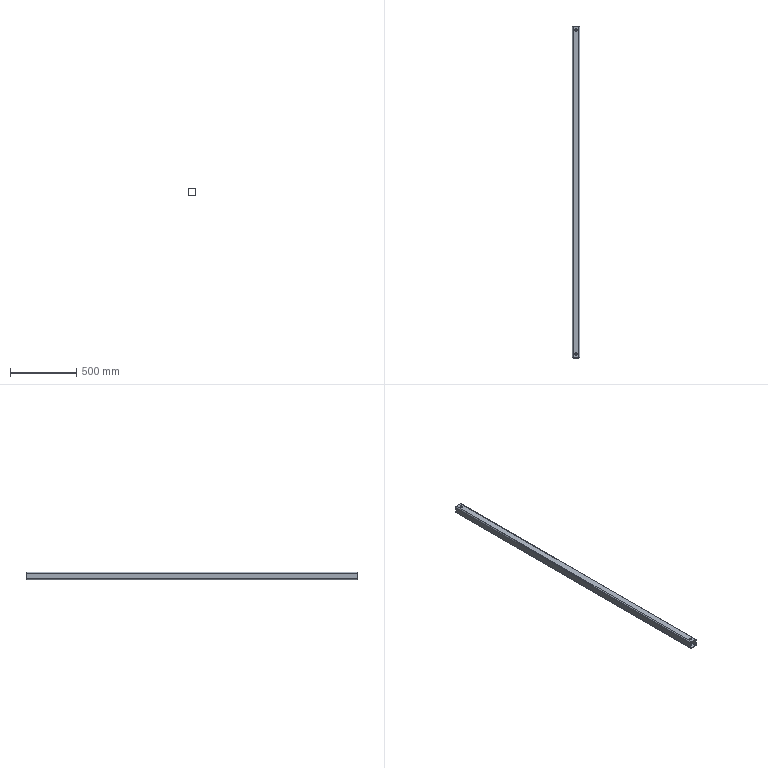Part | SolidWorks | features BaseBody 1 | 1 solid | 26 faces | box 60 x 2500 x 60 mm | volume 2133143 mm3 | cylinder 16 | plane 10 | commonest cylinder face diameters 17.5 x8 8 x4 16 x4
STEP:
#1=CARTESIAN_POINT('',(-678.75,22.,-1300.));
#2=VERTEX_POINT('',#1);
#3=CARTESIAN_POINT('',(-661.25,22.,-1300.));
#4=VERTEX_POINT('',#3);
#5=CARTESIAN_POINT('',(-670.,22.,-1300.));
#6=DIRECTION('',(0.,0.,1.));
#7=DIRECTION('',(-1.,0.,0.));
#8=AXIS2_PLACEMENT_3D('',#5,#6,#7);
#9=CIRCLE('',#8,8.75);
#10=EDGE_CURVE('',#2,#4,#9,.T.);
#11=ORIENTED_EDGE('',*,*,#10,.T.);
#12=CARTESIAN_POINT('',(-661.25,22.,-1304.));
#13=VERTEX_POINT('',#12);
#14=CARTESIAN_POINT('',(-661.25,22.,-1580.));
#15=DIRECTION('',(0.,0.,-1.));
#16=VECTOR('',#15,1000.);
#17=LINE('',#14,#16);
#18=EDGE_CURVE('',#4,#13,#17,.T.);
#19=ORIENTED_EDGE('',*,*,#18,.T.);
#20=CARTESIAN_POINT('',(-678.75,22.,-1304.));
#21=VERTEX_POINT('',#20);
#22=CARTESIAN_POINT('',(-670.,22.,-1304.));
#23=DIRECTION('',(0.,0.,1.));
#24=DIRECTION('',(-1.,0.,0.));
#25=AXIS2_PLACEMENT_3D('',#22,#23,#24);
#26=CIRCLE('',#25,8.75);
#27=EDGE_CURVE('',#21,#13,#26,.T.);
#28=ORIENTED_EDGE('',*,*,#27,.F.);
#29=CARTESIAN_POINT('',(-678.75,22.,-1580.));
#30=DIRECTION('',(0.,0.,-1.));
#31=VECTOR('',#30,1000.);
#32=LINE('',#29,#31);
#33=EDGE_CURVE('',#2,#21,#32,.T.);
#34=ORIENTED_EDGE('',*,*,#33,.F.);
#35=EDGE_LOOP('',(#11,#19,#28,#34));
#36=FACE_OUTER_BOUND('',#35,.T.);
#37=CARTESIAN_POINT('',(-670.,22.,-1580.));
#38=DIRECTION('',(0.,0.,-1.));
#39=DIRECTION('',(-1.,0.,0.));
#40=AXIS2_PLACEMENT_3D('',#37,#38,#39);
#41=CYLINDRICAL_SURFACE('',#40,8.75);
#42=ADVANCED_FACE('',(#36),#41,.F.);
#43=CARTESIAN_POINT('',(-678.75,2462.,-1300.));
#44=VERTEX_POINT('',#43);
#45=CARTESIAN_POINT('',(-661.25,2462.,-1300.));
#46=VERTEX_POINT('',#45);
#47=CARTESIAN_POINT('',(-670.,2462.,-1300.));
#48=DIRECTION('',(0.,0.,1.));
#49=DIRECTION('',(-1.,0.,0.));
#50=AXIS2_PLACEMENT_3D('',#47,#48,#49);
#51=CIRCLE('',#50,8.75);
#52=EDGE_CURVE('',#44,#46,#51,.T.);
#53=ORIENTED_EDGE('',*,*,#52,.T.);
#54=CARTESIAN_POINT('',(-661.25,2462.,-1304.));
#55=VERTEX_POINT('',#54);
#56=CARTESIAN_POINT('',(-661.25,2462.,-1580.));
#57=DIRECTION('',(0.,0.,-1.));
#58=VECTOR('',#57,1000.);
#59=LINE('',#56,#58);
#60=EDGE_CURVE('',#46,#55,#59,.T.);
#61=ORIENTED_EDGE('',*,*,#60,.T.);
#62=CARTESIAN_POINT('',(-678.75,2462.,-1304.));
#63=VERTEX_POINT('',#62);
#64=CARTESIAN_POINT('',(-670.,2462.,-1304.));
#65=DIRECTION('',(0.,0.,1.));
#66=DIRECTION('',(-1.,0.,0.));
#67=AXIS2_PLACEMENT_3D('',#64,#65,#66);
#68=CIRCLE('',#67,8.75);
#69=EDGE_CURVE('',#63,#55,#68,.T.);
#70=ORIENTED_EDGE('',*,*,#69,.F.);
#71=CARTESIAN_POINT('',(-678.75,2462.,-1580.));
#72=DIRECTION('',(0.,0.,-1.));
#73=VECTOR('',#72,1000.);
#74=LINE('',#71,#73);
#75=EDGE_CURVE('',#44,#63,#74,.T.);
#76=ORIENTED_EDGE('',*,*,#75,.F.);
#77=EDGE_LOOP('',(#53,#61,#70,#76));
#78=FACE_OUTER_BOUND('',#77,.T.);
#79=CARTESIAN_POINT('',(-670.,2462.,-1580.));
#80=DIRECTION('',(0.,0.,-1.));
#81=DIRECTION('',(-1.,0.,0.));
#82=AXIS2_PLACEMENT_3D('',#79,#80,#81);
#83=CYLINDRICAL_SURFACE('',#82,8.75);
#84=ADVANCED_FACE('',(#78),#83,.F.);
#85=CARTESIAN_POINT('',(-661.25,22.,-1356.));
#86=VERTEX_POINT('',#85);
#87=CARTESIAN_POINT('',(-678.75,22.,-1356.));
#88=VERTEX_POINT('',#87);
#89=CARTESIAN_POINT('',(-670.,22.,-1356.));
#90=DIRECTION('',(0.,0.,-1.));
#91=DIRECTION('',(-1.,0.,0.));
#92=AXIS2_PLACEMENT_3D('',#89,#90,#91);
#93=CIRCLE('',#92,8.75);
#94=EDGE_CURVE('',#86,#88,#93,.T.);
#95=ORIENTED_EDGE('',*,*,#94,.F.);
#96=CARTESIAN_POINT('',(-661.25,22.,-1360.));
#97=VERTEX_POINT('',#96);
#98=CARTESIAN_POINT('',(-661.25,22.,-1580.));
#99=DIRECTION('',(0.,0.,-1.));
#100=VECTOR('',#99,1000.);
#101=LINE('',#98,#100);
#102=EDGE_CURVE('',#86,#97,#101,.T.);
#103=ORIENTED_EDGE('',*,*,#102,.T.);
#104=CARTESIAN_POINT('',(-678.75,22.,-1360.));
#105=VERTEX_POINT('',#104);
#106=CARTESIAN_POINT('',(-670.,22.,-1360.));
#107=DIRECTION('',(0.,0.,-1.));
#108=DIRECTION('',(-1.,0.,0.));
#109=AXIS2_PLACEMENT_3D('',#106,#107,#108);
#110=CIRCLE('',#109,8.75);
#111=EDGE_CURVE('',#97,#105,#110,.T.);
#112=ORIENTED_EDGE('',*,*,#111,.T.);
#113=CARTESIAN_POINT('',(-678.75,22.,-1580.));
#114=DIRECTION('',(0.,0.,-1.));
#115=VECTOR('',#114,1000.);
#116=LINE('',#113,#115);
#117=EDGE_CURVE('',#88,#105,#116,.T.);
#118=ORIENTED_EDGE('',*,*,#117,.F.);
#119=EDGE_LOOP('',(#95,#103,#112,#118));
#120=FACE_OUTER_BOUND('',#119,.T.);
#121=CARTESIAN_POINT('',(-670.,22.,-1580.));
#122=DIRECTION('',(0.,0.,-1.));
#123=DIRECTION('',(-1.,0.,0.));
#124=AXIS2_PLACEMENT_3D('',#121,#122,#123);
#125=CYLINDRICAL_SURFACE('',#124,8.75);
#126=ADVANCED_FACE('',(#120),#125,.F.);
#127=CARTESIAN_POINT('',(-661.25,2462.,-1356.));
#128=VERTEX_POINT('',#127);
#129=CARTESIAN_POINT('',(-678.75,2462.,-1356.));
#130=VERTEX_POINT('',#129);
#131=CARTESIAN_POINT('',(-670.,2462.,-1356.));
#132=DIRECTION('',(0.,0.,-1.));
#133=DIRECTION('',(-1.,0.,0.));
#134=AXIS2_PLACEMENT_3D('',#131,#132,#133);
#135=CIRCLE('',#134,8.75);
#136=EDGE_CURVE('',#128,#130,#135,.T.);
#137=ORIENTED_EDGE('',*,*,#136,.F.);
#138=CARTESIAN_POINT('',(-661.25,2462.,-1360.));
#139=VERTEX_POINT('',#138);
#140=CARTESIAN_POINT('',(-661.25,2462.,-1580.));
#141=DIRECTION('',(0.,0.,-1.));
#142=VECTOR('',#141,1000.);
#143=LINE('',#140,#142);
#144=EDGE_CURVE('',#128,#139,#143,.T.);
#145=ORIENTED_EDGE('',*,*,#144,.T.);
#146=CARTESIAN_POINT('',(-678.75,2462.,-1360.));
#147=VERTEX_POINT('',#146);
#148=CARTESIAN_POINT('',(-670.,2462.,-1360.));
#149=DIRECTION('',(0.,0.,-1.));
#150=DIRECTION('',(-1.,0.,0.));
#151=AXIS2_PLACEMENT_3D('',#148,#149,#150);
#152=CIRCLE('',#151,8.75);
#153=EDGE_CURVE('',#139,#147,#152,.T.);
#154=ORIENTED_EDGE('',*,*,#153,.T.);
#155=CARTESIAN_POINT('',(-678.75,2462.,-1580.));
#156=DIRECTION('',(0.,0.,-1.));
#157=VECTOR('',#156,1000.);
#158=LINE('',#155,#157);
#159=EDGE_CURVE('',#130,#147,#158,.T.);
#160=ORIENTED_EDGE('',*,*,#159,.F.);
#161=EDGE_LOOP('',(#137,#145,#154,#160));
#162=FACE_OUTER_BOUND('',#161,.T.);
#163=CARTESIAN_POINT('',(-670.,2462.,-1580.));
#164=DIRECTION('',(0.,0.,-1.));
#165=DIRECTION('',(-1.,0.,0.));
#166=AXIS2_PLACEMENT_3D('',#163,#164,#165);
#167=CYLINDRICAL_SURFACE('',#166,8.75);
#168=ADVANCED_FACE('',(#162),#167,.F.);
#169=CARTESIAN_POINT('',(-696.,2492.,-1352.));
#170=VERTEX_POINT('',#169);
#171=CARTESIAN_POINT('',(-696.,2492.,-1308.));
#172=VERTEX_POINT('',#171);
#173=CARTESIAN_POINT('',(-696.,2492.,-1308.));
#174=DIRECTION('',(0.,0.,1.));
#175=VECTOR('',#174,1000.);
#176=LINE('',#173,#175);
#177=EDGE_CURVE('',#170,#172,#176,.T.);
#178=ORIENTED_EDGE('',*,*,#177,.T.);
#179=CARTESIAN_POINT('',(-696.,-8.,-1308.));
#180=VERTEX_POINT('',#179);
#181=CARTESIAN_POINT('',(-696.,22.,-1308.));
#182=DIRECTION('',(0.,-1.,0.));
#183=VECTOR('',#182,1000.);
#184=LINE('',#181,#183);
#185=EDGE_CURVE('',#172,#180,#184,.T.);
#186=ORIENTED_EDGE('',*,*,#185,.T.);
#187=CARTESIAN_POINT('',(-696.,-8.,-1352.));
#188=VERTEX_POINT('',#187);
#189=CARTESIAN_POINT('',(-696.,-8.,-1308.));
#190=DIRECTION('',(0.,0.,-1.));
#191=VECTOR('',#190,1000.);
#192=LINE('',#189,#191);
#193=EDGE_CURVE('',#180,#188,#192,.T.);
#194=ORIENTED_EDGE('',*,*,#193,.T.);
#195=CARTESIAN_POINT('',(-696.,22.,-1352.));
#196=DIRECTION('',(0.,1.,0.));
#197=VECTOR('',#196,1000.);
#198=LINE('',#195,#197);
#199=EDGE_CURVE('',#188,#170,#198,.T.);
#200=ORIENTED_EDGE('',*,*,#199,.T.);
#201=EDGE_LOOP('',(#178,#186,#194,#200));
#202=FACE_OUTER_BOUND('',#201,.T.);
#203=CARTESIAN_POINT('',(-696.,22.,-1308.));
#204=DIRECTION('',(1.,0.,0.));
#205=DIRECTION('',(0.,0.,-1.));
#206=AXIS2_PLACEMENT_3D('',#203,#204,#205);
#207=PLANE('',#206);
#208=ADVANCED_FACE('',(#202),#207,.T.);
#209=ORIENTED_EDGE('',*,*,#185,.F.);
#210=CARTESIAN_POINT('',(-692.,2492.,-1304.));
#211=VERTEX_POINT('',#210);
#212=CARTESIAN_POINT('',(-692.,2492.,-1308.));
#213=DIRECTION('',(0.,-1.,0.));
#214=DIRECTION('',(0.,0.,1.));
#215=AXIS2_PLACEMENT_3D('',#212,#213,#214);
#216=CIRCLE('',#215,4.);
#217=EDGE_CURVE('',#211,#172,#216,.T.);
#218=ORIENTED_EDGE('',*,*,#217,.F.);
#219=CARTESIAN_POINT('',(-692.,-8.,-1304.));
#220=VERTEX_POINT('',#219);
#221=CARTESIAN_POINT('',(-692.,22.,-1304.));
#222=DIRECTION('',(0.,1.,0.));
#223=VECTOR('',#222,1000.);
#224=LINE('',#221,#223);
#225=EDGE_CURVE('',#220,#211,#224,.T.);
#226=ORIENTED_EDGE('',*,*,#225,.F.);
#227=CARTESIAN_POINT('',(-692.,-8.,-1308.));
#228=DIRECTION('',(0.,1.,0.));
#229=DIRECTION('',(0.,0.,1.));
#230=AXIS2_PLACEMENT_3D('',#227,#228,#229);
#231=CIRCLE('',#230,4.);
#232=EDGE_CURVE('',#180,#220,#231,.T.);
#233=ORIENTED_EDGE('',*,*,#232,.F.);
#234=EDGE_LOOP('',(#209,#218,#226,#233));
#235=FACE_OUTER_BOUND('',#234,.T.);
#236=CARTESIAN_POINT('',(-692.,22.,-1308.));
#237=DIRECTION('',(0.,1.,0.));
#238=DIRECTION('',(0.,0.,1.));
#239=AXIS2_PLACEMENT_3D('',#236,#237,#238);
#240=CYLINDRICAL_SURFACE('',#239,4.);
#241=ADVANCED_FACE('',(#235),#240,.F.);
#242=CARTESIAN_POINT('',(-692.,2492.,-1356.));
#243=VERTEX_POINT('',#242);
#244=CARTESIAN_POINT('',(-692.,2492.,-1352.));
#245=DIRECTION('',(0.,-1.,0.));
#246=DIRECTION('',(0.,0.,1.));
#247=AXIS2_PLACEMENT_3D('',#244,#245,#246);
#248=CIRCLE('',#247,4.);
#249=EDGE_CURVE('',#170,#243,#248,.T.);
#250=ORIENTED_EDGE('',*,*,#249,.T.);
#251=CARTESIAN_POINT('',(-648.,2492.,-1356.));
#252=VERTEX_POINT('',#251);
#253=CARTESIAN_POINT('',(-670.,2492.,-1356.));
#254=DIRECTION('',(1.,0.,0.));
#255=VECTOR('',#254,1000.);
#256=LINE('',#253,#255);
#257=EDGE_CURVE('',#243,#252,#256,.T.);
#258=ORIENTED_EDGE('',*,*,#257,.T.);
#259=CARTESIAN_POINT('',(-644.,2492.,-1352.));
#260=VERTEX_POINT('',#259);
#261=CARTESIAN_POINT('',(-648.,2492.,-1352.));
#262=DIRECTION('',(0.,-1.,0.));
#263=DIRECTION('',(0.,0.,1.));
#264=AXIS2_PLACEMENT_3D('',#261,#262,#263);
#265=CIRCLE('',#264,4.);
#266=EDGE_CURVE('',#252,#260,#265,.T.);
#267=ORIENTED_EDGE('',*,*,#266,.T.);
#268=CARTESIAN_POINT('',(-644.,2492.,-1308.));
#269=VERTEX_POINT('',#268);
#270=CARTESIAN_POINT('',(-644.,2492.,-1445.));
#271=DIRECTION('',(0.,0.,1.));
#272=VECTOR('',#271,1000.);
#273=LINE('',#270,#272);
#274=EDGE_CURVE('',#260,#269,#273,.T.);
#275=ORIENTED_EDGE('',*,*,#274,.T.);
#276=CARTESIAN_POINT('',(-648.,2492.,-1304.));
#277=VERTEX_POINT('',#276);
#278=CARTESIAN_POINT('',(-648.,2492.,-1308.));
#279=DIRECTION('',(0.,-1.,0.));
#280=DIRECTION('',(0.,0.,1.));
#281=AXIS2_PLACEMENT_3D('',#278,#279,#280);
#282=CIRCLE('',#281,4.);
#283=EDGE_CURVE('',#269,#277,#282,.T.);
#284=ORIENTED_EDGE('',*,*,#283,.T.);
#285=CARTESIAN_POINT('',(-670.,2492.,-1304.));
#286=DIRECTION('',(-1.,0.,0.));
#287=VECTOR('',#286,1000.);
#288=LINE('',#285,#287);
#289=EDGE_CURVE('',#277,#211,#288,.T.);
#290=ORIENTED_EDGE('',*,*,#289,.T.);
#291=ORIENTED_EDGE('',*,*,#217,.T.);
#292=ORIENTED_EDGE('',*,*,#177,.F.);
#293=EDGE_LOOP('',(#250,#258,#267,#275,#284,#290,#291,#292));
#294=FACE_BOUND('',#293,.T.);
#295=CARTESIAN_POINT('',(-700.,2492.,-1352.));
#296=VERTEX_POINT('',#295);
#297=CARTESIAN_POINT('',(-700.,2492.,-1308.));
#298=VERTEX_POINT('',#297);
#299=CARTESIAN_POINT('',(-700.,2492.,-1445.));
#300=DIRECTION('',(0.,0.,1.));
#301=VECTOR('',#300,1000.);
#302=LINE('',#299,#301);
#303=EDGE_CURVE('',#296,#298,#302,.T.);
#304=ORIENTED_EDGE('',*,*,#303,.T.);
#305=CARTESIAN_POINT('',(-692.,2492.,-1300.));
#306=VERTEX_POINT('',#305);
#307=CARTESIAN_POINT('',(-692.,2492.,-1308.));
#308=DIRECTION('',(0.,1.,0.));
#309=DIRECTION('',(0.,0.,1.));
#310=AXIS2_PLACEMENT_3D('',#307,#308,#309);
#311=CIRCLE('',#310,8.);
#312=EDGE_CURVE('',#298,#306,#311,.T.);
#313=ORIENTED_EDGE('',*,*,#312,.T.);
#314=CARTESIAN_POINT('',(-648.,2492.,-1300.));
#315=VERTEX_POINT('',#314);
#316=CARTESIAN_POINT('',(-670.,2492.,-1300.));
#317=DIRECTION('',(1.,0.,0.));
#318=VECTOR('',#317,1000.);
#319=LINE('',#316,#318);
#320=EDGE_CURVE('',#306,#315,#319,.T.);
#321=ORIENTED_EDGE('',*,*,#320,.T.);
#322=CARTESIAN_POINT('',(-640.,2492.,-1308.));
#323=VERTEX_POINT('',#322);
#324=CARTESIAN_POINT('',(-648.,2492.,-1308.));
#325=DIRECTION('',(0.,1.,0.));
#326=DIRECTION('',(0.,0.,1.));
#327=AXIS2_PLACEMENT_3D('',#324,#325,#326);
#328=CIRCLE('',#327,8.);
#329=EDGE_CURVE('',#315,#323,#328,.T.);
#330=ORIENTED_EDGE('',*,*,#329,.T.);
#331=CARTESIAN_POINT('',(-640.,2492.,-1352.));
#332=VERTEX_POINT('',#331);
#333=CARTESIAN_POINT('',(-640.,2492.,-1445.));
#334=DIRECTION('',(0.,0.,-1.));
#335=VECTOR('',#334,1000.);
#336=LINE('',#333,#335);
#337=EDGE_CURVE('',#323,#332,#336,.T.);
#338=ORIENTED_EDGE('',*,*,#337,.T.);
#339=CARTESIAN_POINT('',(-648.,2492.,-1360.));
#340=VERTEX_POINT('',#339);
#341=CARTESIAN_POINT('',(-648.,2492.,-1352.));
#342=DIRECTION('',(0.,1.,0.));
#343=DIRECTION('',(0.,0.,1.));
#344=AXIS2_PLACEMENT_3D('',#341,#342,#343);
#345=CIRCLE('',#344,8.);
#346=EDGE_CURVE('',#332,#340,#345,.T.);
#347=ORIENTED_EDGE('',*,*,#346,.T.);
#348=CARTESIAN_POINT('',(-692.,2492.,-1360.));
#349=VERTEX_POINT('',#348);
#350=CARTESIAN_POINT('',(-670.,2492.,-1360.));
#351=DIRECTION('',(-1.,0.,0.));
#352=VECTOR('',#351,1000.);
#353=LINE('',#350,#352);
#354=EDGE_CURVE('',#340,#349,#353,.T.);
#355=ORIENTED_EDGE('',*,*,#354,.T.);
#356=CARTESIAN_POINT('',(-692.,2492.,-1352.));
#357=DIRECTION('',(0.,1.,0.));
#358=DIRECTION('',(0.,0.,1.));
#359=AXIS2_PLACEMENT_3D('',#356,#357,#358);
#360=CIRCLE('',#359,8.);
#361=EDGE_CURVE('',#349,#296,#360,.T.);
#362=ORIENTED_EDGE('',*,*,#361,.T.);
#363=EDGE_LOOP('',(#304,#313,#321,#330,#338,#347,#355,#362));
#364=FACE_OUTER_BOUND('',#363,.T.);
#365=CARTESIAN_POINT('',(-670.,2492.,-1445.));
#366=DIRECTION('',(0.,1.,0.));
#367=DIRECTION('',(0.,0.,1.));
#368=AXIS2_PLACEMENT_3D('',#365,#366,#367);
#369=PLANE('',#368);
#370=ADVANCED_FACE('',(#294,#364),#369,.T.);
#371=CARTESIAN_POINT('',(-692.,-8.,-1356.));
#372=VERTEX_POINT('',#371);
#373=CARTESIAN_POINT('',(-692.,22.,-1356.));
#374=DIRECTION('',(0.,-1.,0.));
#375=VECTOR('',#374,1000.);
#376=LINE('',#373,#375);
#377=EDGE_CURVE('',#243,#372,#376,.T.);
#378=ORIENTED_EDGE('',*,*,#377,.F.);
#379=ORIENTED_EDGE('',*,*,#249,.F.);
#380=ORIENTED_EDGE('',*,*,#199,.F.);
#381=CARTESIAN_POINT('',(-692.,-8.,-1352.));
#382=DIRECTION('',(0.,1.,0.));
#383=DIRECTION('',(0.,0.,1.));
#384=AXIS2_PLACEMENT_3D('',#381,#382,#383);
#385=CIRCLE('',#384,4.);
#386=EDGE_CURVE('',#372,#188,#385,.T.);
#387=ORIENTED_EDGE('',*,*,#386,.F.);
#388=EDGE_LOOP('',(#378,#379,#380,#387));
#389=FACE_OUTER_BOUND('',#388,.T.);
#390=CARTESIAN_POINT('',(-692.,22.,-1352.));
#391=DIRECTION('',(0.,1.,0.));
#392=DIRECTION('',(0.,0.,1.));
#393=AXIS2_PLACEMENT_3D('',#390,#391,#392);
#394=CYLINDRICAL_SURFACE('',#393,4.);
#395=ADVANCED_FACE('',(#389),#394,.F.);
#396=CARTESIAN_POINT('',(-644.,-8.,-1352.));
#397=VERTEX_POINT('',#396);
#398=CARTESIAN_POINT('',(-648.,-8.,-1356.));
#399=VERTEX_POINT('',#398);
#400=CARTESIAN_POINT('',(-648.,-8.,-1352.));
#401=DIRECTION('',(0.,1.,0.));
#402=DIRECTION('',(0.,0.,1.));
#403=AXIS2_PLACEMENT_3D('',#400,#401,#402);
#404=CIRCLE('',#403,4.);
#405=EDGE_CURVE('',#397,#399,#404,.T.);
#406=ORIENTED_EDGE('',*,*,#405,.T.);
#407=CARTESIAN_POINT('',(-670.,-8.,-1356.));
#408=DIRECTION('',(-1.,0.,0.));
#409=VECTOR('',#408,1000.);
#410=LINE('',#407,#409);
#411=EDGE_CURVE('',#399,#372,#410,.T.);
#412=ORIENTED_EDGE('',*,*,#411,.T.);
#413=ORIENTED_EDGE('',*,*,#386,.T.);
#414=ORIENTED_EDGE('',*,*,#193,.F.);
#415=ORIENTED_EDGE('',*,*,#232,.T.);
#416=CARTESIAN_POINT('',(-648.,-8.,-1304.));
#417=VERTEX_POINT('',#416);
#418=CARTESIAN_POINT('',(-670.,-8.,-1304.));
#419=DIRECTION('',(1.,0.,0.));
#420=VECTOR('',#419,1000.);
#421=LINE('',#418,#420);
#422=EDGE_CURVE('',#220,#417,#421,.T.);
#423=ORIENTED_EDGE('',*,*,#422,.T.);
#424=CARTESIAN_POINT('',(-644.,-8.,-1308.));
#425=VERTEX_POINT('',#424);
#426=CARTESIAN_POINT('',(-648.,-8.,-1308.));
#427=DIRECTION('',(0.,1.,0.));
#428=DIRECTION('',(0.,0.,1.));
#429=AXIS2_PLACEMENT_3D('',#426,#427,#428);
#430=CIRCLE('',#429,4.);
#431=EDGE_CURVE('',#417,#425,#430,.T.);
#432=ORIENTED_EDGE('',*,*,#431,.T.);
#433=CARTESIAN_POINT('',(-644.,-8.,-1445.));
#434=DIRECTION('',(0.,0.,-1.));
#435=VECTOR('',#434,1000.);
#436=LINE('',#433,#435);
#437=EDGE_CURVE('',#425,#397,#436,.T.);
#438=ORIENTED_EDGE('',*,*,#437,.T.);
#439=EDGE_LOOP('',(#406,#412,#413,#414,#415,#423,#432,#438));
#440=FACE_BOUND('',#439,.T.);
#441=CARTESIAN_POINT('',(-640.,-8.,-1352.));
#442=VERTEX_POINT('',#441);
#443=CARTESIAN_POINT('',(-640.,-8.,-1308.));
#444=VERTEX_POINT('',#443);
#445=CARTESIAN_POINT('',(-640.,-8.,-1445.));
#446=DIRECTION('',(0.,0.,1.));
#447=VECTOR('',#446,1000.);
#448=LINE('',#445,#447);
#449=EDGE_CURVE('',#442,#444,#448,.T.);
#450=ORIENTED_EDGE('',*,*,#449,.T.);
#451=CARTESIAN_POINT('',(-648.,-8.,-1300.));
#452=VERTEX_POINT('',#451);
#453=CARTESIAN_POINT('',(-648.,-8.,-1308.));
#454=DIRECTION('',(0.,-1.,0.));
#455=DIRECTION('',(0.,0.,1.));
#456=AXIS2_PLACEMENT_3D('',#453,#454,#455);
#457=CIRCLE('',#456,8.);
#458=EDGE_CURVE('',#444,#452,#457,.T.);
#459=ORIENTED_EDGE('',*,*,#458,.T.);
#460=CARTESIAN_POINT('',(-692.,-8.,-1300.));
#461=VERTEX_POINT('',#460);
#462=CARTESIAN_POINT('',(-670.,-8.,-1300.));
#463=DIRECTION('',(-1.,0.,0.));
#464=VECTOR('',#463,1000.);
#465=LINE('',#462,#464);
#466=EDGE_CURVE('',#452,#461,#465,.T.);
#467=ORIENTED_EDGE('',*,*,#466,.T.);
#468=CARTESIAN_POINT('',(-700.,-8.,-1308.));
#469=VERTEX_POINT('',#468);
#470=CARTESIAN_POINT('',(-692.,-8.,-1308.));
#471=DIRECTION('',(0.,-1.,0.));
#472=DIRECTION('',(0.,0.,1.));
#473=AXIS2_PLACEMENT_3D('',#470,#471,#472);
#474=CIRCLE('',#473,8.);
#475=EDGE_CURVE('',#461,#469,#474,.T.);
#476=ORIENTED_EDGE('',*,*,#475,.T.);
#477=CARTESIAN_POINT('',(-700.,-8.,-1352.));
#478=VERTEX_POINT('',#477);
#479=CARTESIAN_POINT('',(-700.,-8.,-1445.));
#480=DIRECTION('',(0.,0.,-1.));
#481=VECTOR('',#480,1000.);
#482=LINE('',#479,#481);
#483=EDGE_CURVE('',#469,#478,#482,.T.);
#484=ORIENTED_EDGE('',*,*,#483,.T.);
#485=CARTESIAN_POINT('',(-692.,-8.,-1360.));
#486=VERTEX_POINT('',#485);
#487=CARTESIAN_POINT('',(-692.,-8.,-1352.));
#488=DIRECTION('',(0.,-1.,0.));
#489=DIRECTION('',(0.,0.,1.));
#490=AXIS2_PLACEMENT_3D('',#487,#488,#489);
#491=CIRCLE('',#490,8.);
#492=EDGE_CURVE('',#478,#486,#491,.T.);
#493=ORIENTED_EDGE('',*,*,#492,.T.);
#494=CARTESIAN_POINT('',(-648.,-8.,-1360.));
#495=VERTEX_POINT('',#494);
#496=CARTESIAN_POINT('',(-670.,-8.,-1360.));
#497=DIRECTION('',(1.,0.,0.));
#498=VECTOR('',#497,1000.);
#499=LINE('',#496,#498);
#500=EDGE_CURVE('',#486,#495,#499,.T.);
#501=ORIENTED_EDGE('',*,*,#500,.T.);
#502=CARTESIAN_POINT('',(-648.,-8.,-1352.));
#503=DIRECTION('',(0.,-1.,0.));
#504=DIRECTION('',(0.,0.,1.));
#505=AXIS2_PLACEMENT_3D('',#502,#503,#504);
#506=CIRCLE('',#505,8.);
#507=EDGE_CURVE('',#495,#442,#506,.T.);
#508=ORIENTED_EDGE('',*,*,#507,.T.);
#509=EDGE_LOOP('',(#450,#459,#467,#476,#484,#493,#501,#508));
#510=FACE_OUTER_BOUND('',#509,.T.);
#511=CARTESIAN_POINT('',(-670.,-8.,-1445.));
#512=DIRECTION('',(0.,-1.,0.));
#513=DIRECTION('',(0.,0.,-1.));
#514=AXIS2_PLACEMENT_3D('',#511,#512,#513);
#515=PLANE('',#514);
#516=ADVANCED_FACE('',(#440,#510),#515,.T.);
#517=ORIENTED_EDGE('',*,*,#27,.T.);
#518=CARTESIAN_POINT('',(-670.,22.,-1304.));
#519=DIRECTION('',(0.,0.,1.));
#520=DIRECTION('',(-1.,0.,0.));
#521=AXIS2_PLACEMENT_3D('',#518,#519,#520);
#522=CIRCLE('',#521,8.75);
#523=EDGE_CURVE('',#13,#21,#522,.T.);
#524=ORIENTED_EDGE('',*,*,#523,.T.);
#525=EDGE_LOOP('',(#517,#524));
#526=FACE_BOUND('',#525,.T.);
#527=ORIENTED_EDGE('',*,*,#69,.T.);
#528=CARTESIAN_POINT('',(-670.,2462.,-1304.));
#529=DIRECTION('',(0.,0.,1.));
#530=DIRECTION('',(-1.,0.,0.));
#531=AXIS2_PLACEMENT_3D('',#528,#529,#530);
#532=CIRCLE('',#531,8.75);
#533=EDGE_CURVE('',#55,#63,#532,.T.);
#534=ORIENTED_EDGE('',*,*,#533,.T.);
#535=EDGE_LOOP('',(#527,#534));
#536=FACE_BOUND('',#535,.T.);
#537=ORIENTED_EDGE('',*,*,#289,.F.);
#538=CARTESIAN_POINT('',(-648.,22.,-1304.));
#539=DIRECTION('',(0.,-1.,0.));
#540=VECTOR('',#539,1000.);
#541=LINE('',#538,#540);
#542=EDGE_CURVE('',#277,#417,#541,.T.);
#543=ORIENTED_EDGE('',*,*,#542,.T.);
#544=ORIENTED_EDGE('',*,*,#422,.F.);
#545=ORIENTED_EDGE('',*,*,#225,.T.);
#546=EDGE_LOOP('',(#537,#543,#544,#545));
#547=FACE_OUTER_BOUND('',#546,.T.);
#548=CARTESIAN_POINT('',(-692.,22.,-1304.));
#549=DIRECTION('',(0.,0.,-1.));
#550=DIRECTION('',(-1.,0.,0.));
#551=AXIS2_PLACEMENT_3D('',#548,#549,#550);
#552=PLANE('',#551);
#553=ADVANCED_FACE('',(#526,#536,#547),#552,.T.);
#554=CARTESIAN_POINT('',(-670.,22.,-1356.));
#555=DIRECTION('',(0.,0.,-1.));
#556=DIRECTION('',(-1.,0.,0.));
#557=AXIS2_PLACEMENT_3D('',#554,#555,#556);
#558=CIRCLE('',#557,8.75);
#559=EDGE_CURVE('',#88,#86,#558,.T.);
#560=ORIENTED_EDGE('',*,*,#559,.T.);
#561=ORIENTED_EDGE('',*,*,#94,.T.);
#562=EDGE_LOOP('',(#560,#561));
#563=FACE_BOUND('',#562,.T.);
#564=CARTESIAN_POINT('',(-670.,2462.,-1356.));
#565=DIRECTION('',(0.,0.,-1.));
#566=DIRECTION('',(-1.,0.,0.));
#567=AXIS2_PLACEMENT_3D('',#564,#565,#566);
#568=CIRCLE('',#567,8.75);
#569=EDGE_CURVE('',#130,#128,#568,.T.);
#570=ORIENTED_EDGE('',*,*,#569,.T.);
#571=ORIENTED_EDGE('',*,*,#136,.T.);
#572=EDGE_LOOP('',(#570,#571));
#573=FACE_BOUND('',#572,.T.);
#574=ORIENTED_EDGE('',*,*,#257,.F.);
#575=ORIENTED_EDGE('',*,*,#377,.T.);
#576=ORIENTED_EDGE('',*,*,#411,.F.);
#577=CARTESIAN_POINT('',(-648.,22.,-1356.));
#578=DIRECTION('',(0.,1.,0.));
#579=VECTOR('',#578,1000.);
#580=LINE('',#577,#579);
#581=EDGE_CURVE('',#399,#252,#580,.T.);
#582=ORIENTED_EDGE('',*,*,#581,.T.);
#583=EDGE_LOOP('',(#574,#575,#576,#582));
#584=FACE_OUTER_BOUND('',#583,.T.);
#585=CARTESIAN_POINT('',(-648.,22.,-1356.));
#586=DIRECTION('',(0.,0.,1.));
#587=DIRECTION('',(1.,0.,0.));
#588=AXIS2_PLACEMENT_3D('',#585,#586,#587);
#589=PLANE('',#588);
#590=ADVANCED_FACE('',(#563,#573,#584),#589,.T.);
#591=ORIENTED_EDGE('',*,*,#542,.F.);
#592=ORIENTED_EDGE('',*,*,#283,.F.);
#593=CARTESIAN_POINT('',(-644.,22.,-1308.));
#594=DIRECTION('',(0.,1.,0.));
#595=VECTOR('',#594,1000.);
#596=LINE('',#593,#595);
#597=EDGE_CURVE('',#425,#269,#596,.T.);
#598=ORIENTED_EDGE('',*,*,#597,.F.);
#599=ORIENTED_EDGE('',*,*,#431,.F.);
#600=EDGE_LOOP('',(#591,#592,#598,#599));
#601=FACE_OUTER_BOUND('',#600,.T.);
#602=CARTESIAN_POINT('',(-648.,22.,-1308.));
#603=DIRECTION('',(0.,1.,0.));
#604=DIRECTION('',(0.,0.,1.));
#605=AXIS2_PLACEMENT_3D('',#602,#603,#604);
#606=CYLINDRICAL_SURFACE('',#605,4.);
#607=ADVANCED_FACE('',(#601),#606,.F.);
#608=ORIENTED_EDGE('',*,*,#274,.F.);
#609=CARTESIAN_POINT('',(-644.,22.,-1352.));
#610=DIRECTION('',(0.,-1.,0.));
#611=VECTOR('',#610,1000.);
#612=LINE('',#609,#611);
#613=EDGE_CURVE('',#260,#397,#612,.T.);
#614=ORIENTED_EDGE('',*,*,#613,.T.);
#615=ORIENTED_EDGE('',*,*,#437,.F.);
#616=ORIENTED_EDGE('',*,*,#597,.T.);
#617=EDGE_LOOP('',(#608,#614,#615,#616));
#618=FACE_OUTER_BOUND('',#617,.T.);
#619=CARTESIAN_POINT('',(-644.,22.,-1352.));
#620=DIRECTION('',(-1.,0.,0.));
#621=DIRECTION('',(0.,0.,1.));
#622=AXIS2_PLACEMENT_3D('',#619,#620,#621);
#623=PLANE('',#622);
#624=ADVANCED_FACE('',(#618),#623,.T.);
#625=ORIENTED_EDGE('',*,*,#613,.F.);
#626=ORIENTED_EDGE('',*,*,#266,.F.);
#627=ORIENTED_EDGE('',*,*,#581,.F.);
#628=ORIENTED_EDGE('',*,*,#405,.F.);
#629=EDGE_LOOP('',(#625,#626,#627,#628));
#630=FACE_OUTER_BOUND('',#629,.T.);
#631=CARTESIAN_POINT('',(-648.,22.,-1352.));
#632=DIRECTION('',(0.,1.,0.));
#633=DIRECTION('',(0.,0.,1.));
#634=AXIS2_PLACEMENT_3D('',#631,#632,#633);
#635=CYLINDRICAL_SURFACE('',#634,4.);
#636=ADVANCED_FACE('',(#630),#635,.F.);
#637=ORIENTED_EDGE('',*,*,#312,.F.);
#638=CARTESIAN_POINT('',(-700.,22.,-1308.));
#639=DIRECTION('',(0.,-1.,0.));
#640=VECTOR('',#639,1000.);
#641=LINE('',#638,#640);
#642=EDGE_CURVE('',#298,#469,#641,.T.);
#643=ORIENTED_EDGE('',*,*,#642,.T.);
#644=ORIENTED_EDGE('',*,*,#475,.F.);
#645=CARTESIAN_POINT('',(-692.,22.,-1300.));
#646=DIRECTION('',(0.,1.,0.));
#647=VECTOR('',#646,1000.);
#648=LINE('',#645,#647);
#649=EDGE_CURVE('',#461,#306,#648,.T.);
#650=ORIENTED_EDGE('',*,*,#649,.T.);
#651=EDGE_LOOP('',(#637,#643,#644,#650));
#652=FACE_OUTER_BOUND('',#651,.T.);
#653=CARTESIAN_POINT('',(-692.,22.,-1308.));
#654=DIRECTION('',(0.,1.,0.));
#655=DIRECTION('',(0.,0.,1.));
#656=AXIS2_PLACEMENT_3D('',#653,#654,#655);
#657=CYLINDRICAL_SURFACE('',#656,8.);
#658=ADVANCED_FACE('',(#652),#657,.T.);
#659=ORIENTED_EDGE('',*,*,#642,.F.);
#660=ORIENTED_EDGE('',*,*,#303,.F.);
#661=CARTESIAN_POINT('',(-700.,22.,-1352.));
#662=DIRECTION('',(0.,1.,0.));
#663=VECTOR('',#662,1000.);
#664=LINE('',#661,#663);
#665=EDGE_CURVE('',#478,#296,#664,.T.);
#666=ORIENTED_EDGE('',*,*,#665,.F.);
#667=ORIENTED_EDGE('',*,*,#483,.F.);
#668=EDGE_LOOP('',(#659,#660,#666,#667));
#669=FACE_OUTER_BOUND('',#668,.T.);
#670=CARTESIAN_POINT('',(-700.,22.,-1308.));
#671=DIRECTION('',(1.,0.,0.));
#672=DIRECTION('',(0.,0.,-1.));
#673=AXIS2_PLACEMENT_3D('',#670,#671,#672);
#674=PLANE('',#673);
#675=ADVANCED_FACE('',(#669),#674,.F.);
#676=ORIENTED_EDGE('',*,*,#361,.F.);
#677=CARTESIAN_POINT('',(-692.,22.,-1360.));
#678=DIRECTION('',(0.,-1.,0.));
#679=VECTOR('',#678,1000.);
#680=LINE('',#677,#679);
#681=EDGE_CURVE('',#349,#486,#680,.T.);
#682=ORIENTED_EDGE('',*,*,#681,.T.);
#683=ORIENTED_EDGE('',*,*,#492,.F.);
#684=ORIENTED_EDGE('',*,*,#665,.T.);
#685=EDGE_LOOP('',(#676,#682,#683,#684));
#686=FACE_OUTER_BOUND('',#685,.T.);
#687=CARTESIAN_POINT('',(-692.,22.,-1352.));
#688=DIRECTION('',(0.,1.,0.));
#689=DIRECTION('',(0.,0.,1.));
#690=AXIS2_PLACEMENT_3D('',#687,#688,#689);
#691=CYLINDRICAL_SURFACE('',#690,8.);
#692=ADVANCED_FACE('',(#686),#691,.T.);
#693=CARTESIAN_POINT('',(-670.,22.,-1360.));
#694=DIRECTION('',(0.,0.,-1.));
#695=DIRECTION('',(-1.,0.,0.));
#696=AXIS2_PLACEMENT_3D('',#693,#694,#695);
#697=CIRCLE('',#696,8.75);
#698=EDGE_CURVE('',#105,#97,#697,.T.);
#699=ORIENTED_EDGE('',*,*,#698,.F.);
#700=ORIENTED_EDGE('',*,*,#111,.F.);
#701=EDGE_LOOP('',(#699,#700));
#702=FACE_BOUND('',#701,.T.);
#703=CARTESIAN_POINT('',(-670.,2462.,-1360.));
#704=DIRECTION('',(0.,0.,-1.));
#705=DIRECTION('',(-1.,0.,0.));
#706=AXIS2_PLACEMENT_3D('',#703,#704,#705);
#707=CIRCLE('',#706,8.75);
#708=EDGE_CURVE('',#147,#139,#707,.T.);
#709=ORIENTED_EDGE('',*,*,#708,.F.);
#710=ORIENTED_EDGE('',*,*,#153,.F.);
#711=EDGE_LOOP('',(#709,#710));
#712=FACE_BOUND('',#711,.T.);
#713=ORIENTED_EDGE('',*,*,#681,.F.);
#714=ORIENTED_EDGE('',*,*,#354,.F.);
#715=CARTESIAN_POINT('',(-648.,22.,-1360.));
#716=DIRECTION('',(0.,1.,0.));
#717=VECTOR('',#716,1000.);
#718=LINE('',#715,#717);
#719=EDGE_CURVE('',#495,#340,#718,.T.);
#720=ORIENTED_EDGE('',*,*,#719,.F.);
#721=ORIENTED_EDGE('',*,*,#500,.F.);
#722=EDGE_LOOP('',(#713,#714,#720,#721));
#723=FACE_OUTER_BOUND('',#722,.T.);
#724=CARTESIAN_POINT('',(-648.,22.,-1360.));
#725=DIRECTION('',(0.,0.,1.));
#726=DIRECTION('',(1.,0.,0.));
#727=AXIS2_PLACEMENT_3D('',#724,#725,#726);
#728=PLANE('',#727);
#729=ADVANCED_FACE('',(#702,#712,#723),#728,.F.);
#730=ORIENTED_EDGE('',*,*,#346,.F.);
#731=CARTESIAN_POINT('',(-640.,22.,-1352.));
#732=DIRECTION('',(0.,-1.,0.));
#733=VECTOR('',#732,1000.);
#734=LINE('',#731,#733);
#735=EDGE_CURVE('',#332,#442,#734,.T.);
#736=ORIENTED_EDGE('',*,*,#735,.T.);
#737=ORIENTED_EDGE('',*,*,#507,.F.);
#738=ORIENTED_EDGE('',*,*,#719,.T.);
#739=EDGE_LOOP('',(#730,#736,#737,#738));
#740=FACE_OUTER_BOUND('',#739,.T.);
#741=CARTESIAN_POINT('',(-648.,22.,-1352.));
#742=DIRECTION('',(0.,1.,0.));
#743=DIRECTION('',(0.,0.,1.));
#744=AXIS2_PLACEMENT_3D('',#741,#742,#743);
#745=CYLINDRICAL_SURFACE('',#744,8.);
#746=ADVANCED_FACE('',(#740),#745,.T.);
#747=ORIENTED_EDGE('',*,*,#735,.F.);
#748=ORIENTED_EDGE('',*,*,#337,.F.);
#749=CARTESIAN_POINT('',(-640.,22.,-1308.));
#750=DIRECTION('',(0.,1.,0.));
#751=VECTOR('',#750,1000.);
#752=LINE('',#749,#751);
#753=EDGE_CURVE('',#444,#323,#752,.T.);
#754=ORIENTED_EDGE('',*,*,#753,.F.);
#755=ORIENTED_EDGE('',*,*,#449,.F.);
#756=EDGE_LOOP('',(#747,#748,#754,#755));
#757=FACE_OUTER_BOUND('',#756,.T.);
#758=CARTESIAN_POINT('',(-640.,22.,-1352.));
#759=DIRECTION('',(-1.,0.,0.));
#760=DIRECTION('',(0.,0.,1.));
#761=AXIS2_PLACEMENT_3D('',#758,#759,#760);
#762=PLANE('',#761);
#763=ADVANCED_FACE('',(#757),#762,.F.);
#764=ORIENTED_EDGE('',*,*,#329,.F.);
#765=CARTESIAN_POINT('',(-648.,22.,-1300.));
#766=DIRECTION('',(0.,-1.,0.));
#767=VECTOR('',#766,1000.);
#768=LINE('',#765,#767);
#769=EDGE_CURVE('',#315,#452,#768,.T.);
#770=ORIENTED_EDGE('',*,*,#769,.T.);
#771=ORIENTED_EDGE('',*,*,#458,.F.);
#772=ORIENTED_EDGE('',*,*,#753,.T.);
#773=EDGE_LOOP('',(#764,#770,#771,#772));
#774=FACE_OUTER_BOUND('',#773,.T.);
#775=CARTESIAN_POINT('',(-648.,22.,-1308.));
#776=DIRECTION('',(0.,1.,0.));
#777=DIRECTION('',(0.,0.,1.));
#778=AXIS2_PLACEMENT_3D('',#775,#776,#777);
#779=CYLINDRICAL_SURFACE('',#778,8.);
#780=ADVANCED_FACE('',(#774),#779,.T.);
#781=ORIENTED_EDGE('',*,*,#10,.F.);
#782=CARTESIAN_POINT('',(-670.,22.,-1300.));
#783=DIRECTION('',(0.,0.,1.));
#784=DIRECTION('',(-1.,0.,0.));
#785=AXIS2_PLACEMENT_3D('',#782,#783,#784);
#786=CIRCLE('',#785,8.75);
#787=EDGE_CURVE('',#4,#2,#786,.T.);
#788=ORIENTED_EDGE('',*,*,#787,.F.);
#789=EDGE_LOOP('',(#781,#788));
#790=FACE_BOUND('',#789,.T.);
#791=ORIENTED_EDGE('',*,*,#52,.F.);
#792=CARTESIAN_POINT('',(-670.,2462.,-1300.));
#793=DIRECTION('',(0.,0.,1.));
#794=DIRECTION('',(-1.,0.,0.));
#795=AXIS2_PLACEMENT_3D('',#792,#793,#794);
#796=CIRCLE('',#795,8.75);
#797=EDGE_CURVE('',#46,#44,#796,.T.);
#798=ORIENTED_EDGE('',*,*,#797,.F.);
#799=EDGE_LOOP('',(#791,#798));
#800=FACE_BOUND('',#799,.T.);
#801=ORIENTED_EDGE('',*,*,#769,.F.);
#802=ORIENTED_EDGE('',*,*,#320,.F.);
#803=ORIENTED_EDGE('',*,*,#649,.F.);
#804=ORIENTED_EDGE('',*,*,#466,.F.);
#805=EDGE_LOOP('',(#801,#802,#803,#804));
#806=FACE_OUTER_BOUND('',#805,.T.);
#807=CARTESIAN_POINT('',(-692.,22.,-1300.));
#808=DIRECTION('',(0.,0.,-1.));
#809=DIRECTION('',(-1.,0.,0.));
#810=AXIS2_PLACEMENT_3D('',#807,#808,#809);
#811=PLANE('',#810);
#812=ADVANCED_FACE('',(#790,#800,#806),#811,.F.);
#813=ORIENTED_EDGE('',*,*,#18,.F.);
#814=ORIENTED_EDGE('',*,*,#787,.T.);
#815=ORIENTED_EDGE('',*,*,#33,.T.);
#816=ORIENTED_EDGE('',*,*,#523,.F.);
#817=EDGE_LOOP('',(#813,#814,#815,#816));
#818=FACE_OUTER_BOUND('',#817,.T.);
#819=CARTESIAN_POINT('',(-670.,22.,-1580.));
#820=DIRECTION('',(0.,0.,-1.));
#821=DIRECTION('',(-1.,0.,0.));
#822=AXIS2_PLACEMENT_3D('',#819,#820,#821);
#823=CYLINDRICAL_SURFACE('',#822,8.75);
#824=ADVANCED_FACE('',(#818),#823,.F.);
#825=ORIENTED_EDGE('',*,*,#60,.F.);
#826=ORIENTED_EDGE('',*,*,#797,.T.);
#827=ORIENTED_EDGE('',*,*,#75,.T.);
#828=ORIENTED_EDGE('',*,*,#533,.F.);
#829=EDGE_LOOP('',(#825,#826,#827,#828));
#830=FACE_OUTER_BOUND('',#829,.T.);
#831=CARTESIAN_POINT('',(-670.,2462.,-1580.));
#832=DIRECTION('',(0.,0.,-1.));
#833=DIRECTION('',(-1.,0.,0.));
#834=AXIS2_PLACEMENT_3D('',#831,#832,#833);
#835=CYLINDRICAL_SURFACE('',#834,8.75);
#836=ADVANCED_FACE('',(#830),#835,.F.);
#837=ORIENTED_EDGE('',*,*,#102,.F.);
#838=ORIENTED_EDGE('',*,*,#559,.F.);
#839=ORIENTED_EDGE('',*,*,#117,.T.);
#840=ORIENTED_EDGE('',*,*,#698,.T.);
#841=EDGE_LOOP('',(#837,#838,#839,#840));
#842=FACE_OUTER_BOUND('',#841,.T.);
#843=CARTESIAN_POINT('',(-670.,22.,-1580.));
#844=DIRECTION('',(0.,0.,-1.));
#845=DIRECTION('',(-1.,0.,0.));
#846=AXIS2_PLACEMENT_3D('',#843,#844,#845);
#847=CYLINDRICAL_SURFACE('',#846,8.75);
#848=ADVANCED_FACE('',(#842),#847,.F.);
#849=ORIENTED_EDGE('',*,*,#144,.F.);
#850=ORIENTED_EDGE('',*,*,#569,.F.);
#851=ORIENTED_EDGE('',*,*,#159,.T.);
#852=ORIENTED_EDGE('',*,*,#708,.T.);
#853=EDGE_LOOP('',(#849,#850,#851,#852));
#854=FACE_OUTER_BOUND('',#853,.T.);
#855=CARTESIAN_POINT('',(-670.,2462.,-1580.));
#856=DIRECTION('',(0.,0.,-1.));
#857=DIRECTION('',(-1.,0.,0.));
#858=AXIS2_PLACEMENT_3D('',#855,#856,#857);
#859=CYLINDRICAL_SURFACE('',#858,8.75);
#860=ADVANCED_FACE('',(#854),#859,.F.);
#861=CLOSED_SHELL('',(#42,#84,#126,#168,#208,#241,#370,#395,#516,#553,#590,#607,#624,#636,#658,#675,#692,#729,#746,#763,#780,#812,#824,#836,#848,#860));
#862=MANIFOLD_SOLID_BREP('',#861);
#863=CARTESIAN_POINT('',(0.,0.,0.));
#864=DIRECTION('',(0.,0.,1.));
#865=DIRECTION('',(1.,0.,0.));
#866=AXIS2_PLACEMENT_3D('',#863,#864,#865);
#867=(LENGTH_UNIT()NAMED_UNIT(*)SI_UNIT(.MILLI.,.METRE.));
#868=UNCERTAINTY_MEASURE_WITH_UNIT(LENGTH_MEASURE(0.00001),#867,'','');
#869=(NAMED_UNIT(*)PLANE_ANGLE_UNIT()SI_UNIT($,.RADIAN.));
#870=(NAMED_UNIT(*)SI_UNIT($,.STERADIAN.)SOLID_ANGLE_UNIT());
#871=(GEOMETRIC_REPRESENTATION_CONTEXT(3)GLOBAL_UNCERTAINTY_ASSIGNED_CONTEXT((#868))GLOBAL_UNIT_ASSIGNED_CONTEXT((#867,#869,#870))REPRESENTATION_CONTEXT('',''));
#872=ADVANCED_BREP_SHAPE_REPRESENTATION('',(#862,#866),#871);